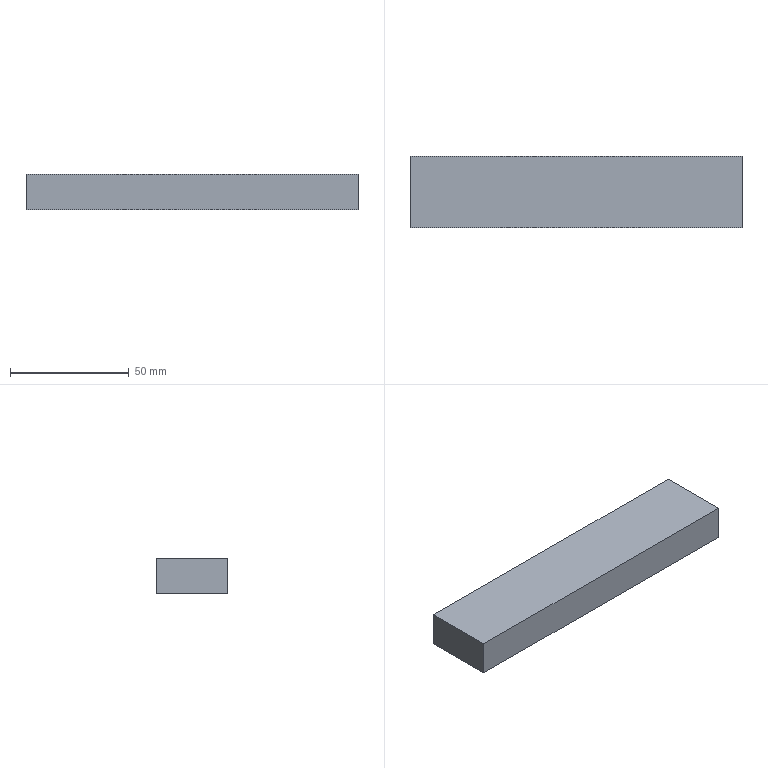Part | NX | features solid 2 | 1 solid | 6 faces | box 140 x 30 x 15 mm | volume 63000 mm3 | plane 6
STEP:
#1=CARTESIAN_POINT('',(-512.5,50.,-100.));
#2=VERTEX_POINT('',#1);
#3=CARTESIAN_POINT('',(-512.5,80.,-100.));
#4=VERTEX_POINT('',#3);
#5=CARTESIAN_POINT('',(-512.5,50.,-100.));
#6=DIRECTION('',(0.,-1.,0.));
#7=VECTOR('',#6,1000.);
#8=LINE('',#5,#7);
#9=EDGE_CURVE('',#2,#4,#8,.F.);
#10=ORIENTED_EDGE('',*,*,#9,.F.);
#11=CARTESIAN_POINT('',(-512.5,50.,-85.));
#12=VERTEX_POINT('',#11);
#13=CARTESIAN_POINT('',(-512.5,50.,-100.));
#14=DIRECTION('',(0.,0.,1.));
#15=VECTOR('',#14,1000.);
#16=LINE('',#13,#15);
#17=EDGE_CURVE('',#2,#12,#16,.T.);
#18=ORIENTED_EDGE('',*,*,#17,.T.);
#19=CARTESIAN_POINT('',(-512.5,80.,-85.));
#20=VERTEX_POINT('',#19);
#21=CARTESIAN_POINT('',(-512.5,40.,-85.));
#22=DIRECTION('',(0.,1.,0.));
#23=VECTOR('',#22,1000.);
#24=LINE('',#21,#23);
#25=EDGE_CURVE('',#12,#20,#24,.T.);
#26=ORIENTED_EDGE('',*,*,#25,.T.);
#27=CARTESIAN_POINT('',(-512.5,80.,-100.));
#28=DIRECTION('',(0.,0.,1.));
#29=VECTOR('',#28,1000.);
#30=LINE('',#27,#29);
#31=EDGE_CURVE('',#4,#20,#30,.T.);
#32=ORIENTED_EDGE('',*,*,#31,.F.);
#33=EDGE_LOOP('',(#10,#18,#26,#32));
#34=FACE_BOUND('',#33,.T.);
#35=CARTESIAN_POINT('',(-512.5,40.,-115.));
#36=DIRECTION('',(-1.,0.,0.));
#37=DIRECTION('',(0.,0.,1.));
#38=AXIS2_PLACEMENT_3D('',#35,#36,#37);
#39=PLANE('',#38);
#40=ADVANCED_FACE('',(#34),#39,.T.);
#41=ORIENTED_EDGE('',*,*,#25,.F.);
#42=CARTESIAN_POINT('',(-372.5,50.,-85.));
#43=VERTEX_POINT('',#42);
#44=CARTESIAN_POINT('',(-442.5,50.,-85.));
#45=DIRECTION('',(1.,0.,0.));
#46=VECTOR('',#45,1000.);
#47=LINE('',#44,#46);
#48=EDGE_CURVE('',#12,#43,#47,.T.);
#49=ORIENTED_EDGE('',*,*,#48,.T.);
#50=CARTESIAN_POINT('',(-372.5,80.,-85.));
#51=VERTEX_POINT('',#50);
#52=CARTESIAN_POINT('',(-372.5,50.,-85.));
#53=DIRECTION('',(0.,-1.,0.));
#54=VECTOR('',#53,1000.);
#55=LINE('',#52,#54);
#56=EDGE_CURVE('',#43,#51,#55,.F.);
#57=ORIENTED_EDGE('',*,*,#56,.T.);
#58=CARTESIAN_POINT('',(-442.5,80.,-85.));
#59=DIRECTION('',(1.,0.,0.));
#60=VECTOR('',#59,1000.);
#61=LINE('',#58,#60);
#62=EDGE_CURVE('',#20,#51,#61,.T.);
#63=ORIENTED_EDGE('',*,*,#62,.F.);
#64=EDGE_LOOP('',(#41,#49,#57,#63));
#65=FACE_BOUND('',#64,.T.);
#66=CARTESIAN_POINT('',(-442.5,50.,-85.));
#67=DIRECTION('',(0.,0.,1.));
#68=DIRECTION('',(1.,0.,0.));
#69=AXIS2_PLACEMENT_3D('',#66,#67,#68);
#70=PLANE('',#69);
#71=ADVANCED_FACE('',(#65),#70,.T.);
#72=ORIENTED_EDGE('',*,*,#56,.F.);
#73=CARTESIAN_POINT('',(-372.5,50.,-100.));
#74=VERTEX_POINT('',#73);
#75=CARTESIAN_POINT('',(-372.5,50.,-85.));
#76=DIRECTION('',(0.,0.,-1.));
#77=VECTOR('',#76,1000.);
#78=LINE('',#75,#77);
#79=EDGE_CURVE('',#74,#43,#78,.F.);
#80=ORIENTED_EDGE('',*,*,#79,.F.);
#81=CARTESIAN_POINT('',(-372.5,80.,-100.));
#82=VERTEX_POINT('',#81);
#83=CARTESIAN_POINT('',(-372.5,50.,-100.));
#84=DIRECTION('',(0.,1.,0.));
#85=VECTOR('',#84,1000.);
#86=LINE('',#83,#85);
#87=EDGE_CURVE('',#74,#82,#86,.T.);
#88=ORIENTED_EDGE('',*,*,#87,.T.);
#89=CARTESIAN_POINT('',(-372.5,80.,-85.));
#90=DIRECTION('',(0.,0.,-1.));
#91=VECTOR('',#90,1000.);
#92=LINE('',#89,#91);
#93=EDGE_CURVE('',#82,#51,#92,.F.);
#94=ORIENTED_EDGE('',*,*,#93,.T.);
#95=EDGE_LOOP('',(#72,#80,#88,#94));
#96=FACE_BOUND('',#95,.T.);
#97=CARTESIAN_POINT('',(-372.5,50.,-85.));
#98=DIRECTION('',(-1.,0.,0.));
#99=DIRECTION('',(0.,0.,1.));
#100=AXIS2_PLACEMENT_3D('',#97,#98,#99);
#101=PLANE('',#100);
#102=ADVANCED_FACE('',(#96),#101,.F.);
#103=CARTESIAN_POINT('',(-442.5,50.,-100.));
#104=DIRECTION('',(1.,0.,0.));
#105=VECTOR('',#104,1000.);
#106=LINE('',#103,#105);
#107=EDGE_CURVE('',#2,#74,#106,.T.);
#108=ORIENTED_EDGE('',*,*,#107,.F.);
#109=ORIENTED_EDGE('',*,*,#9,.T.);
#110=CARTESIAN_POINT('',(-442.5,80.,-100.));
#111=DIRECTION('',(1.,0.,0.));
#112=VECTOR('',#111,1000.);
#113=LINE('',#110,#112);
#114=EDGE_CURVE('',#4,#82,#113,.T.);
#115=ORIENTED_EDGE('',*,*,#114,.T.);
#116=ORIENTED_EDGE('',*,*,#87,.F.);
#117=EDGE_LOOP('',(#108,#109,#115,#116));
#118=FACE_BOUND('',#117,.T.);
#119=CARTESIAN_POINT('',(-442.5,50.,-100.));
#120=DIRECTION('',(0.,0.,1.));
#121=DIRECTION('',(1.,0.,0.));
#122=AXIS2_PLACEMENT_3D('',#119,#120,#121);
#123=PLANE('',#122);
#124=ADVANCED_FACE('',(#118),#123,.F.);
#125=ORIENTED_EDGE('',*,*,#93,.F.);
#126=ORIENTED_EDGE('',*,*,#114,.F.);
#127=ORIENTED_EDGE('',*,*,#31,.T.);
#128=ORIENTED_EDGE('',*,*,#62,.T.);
#129=EDGE_LOOP('',(#125,#126,#127,#128));
#130=FACE_BOUND('',#129,.T.);
#131=CARTESIAN_POINT('',(-442.5,80.,-100.));
#132=DIRECTION('',(0.,1.,0.));
#133=DIRECTION('',(0.,0.,1.));
#134=AXIS2_PLACEMENT_3D('',#131,#132,#133);
#135=PLANE('',#134);
#136=ADVANCED_FACE('',(#130),#135,.T.);
#137=ORIENTED_EDGE('',*,*,#79,.T.);
#138=ORIENTED_EDGE('',*,*,#48,.F.);
#139=ORIENTED_EDGE('',*,*,#17,.F.);
#140=ORIENTED_EDGE('',*,*,#107,.T.);
#141=EDGE_LOOP('',(#137,#138,#139,#140));
#142=FACE_BOUND('',#141,.T.);
#143=CARTESIAN_POINT('',(-442.5,50.,-100.));
#144=DIRECTION('',(0.,1.,0.));
#145=DIRECTION('',(0.,0.,1.));
#146=AXIS2_PLACEMENT_3D('',#143,#144,#145);
#147=PLANE('',#146);
#148=ADVANCED_FACE('',(#142),#147,.F.);
#149=CLOSED_SHELL('',(#40,#71,#102,#124,#136,#148));
#150=MANIFOLD_SOLID_BREP('',#149);
#151=(LENGTH_UNIT()NAMED_UNIT(*)SI_UNIT(.MILLI.,.METRE.));
#152=UNCERTAINTY_MEASURE_WITH_UNIT(LENGTH_MEASURE(0.00001),#151,'','');
#153=(NAMED_UNIT(*)PLANE_ANGLE_UNIT()SI_UNIT($,.RADIAN.));
#154=(NAMED_UNIT(*)SI_UNIT($,.STERADIAN.)SOLID_ANGLE_UNIT());
#155=(GEOMETRIC_REPRESENTATION_CONTEXT(3)GLOBAL_UNCERTAINTY_ASSIGNED_CONTEXT((#152))GLOBAL_UNIT_ASSIGNED_CONTEXT((#151,#153,#154))REPRESENTATION_CONTEXT('',''));
#156=ADVANCED_BREP_SHAPE_REPRESENTATION('',(#150),#155);